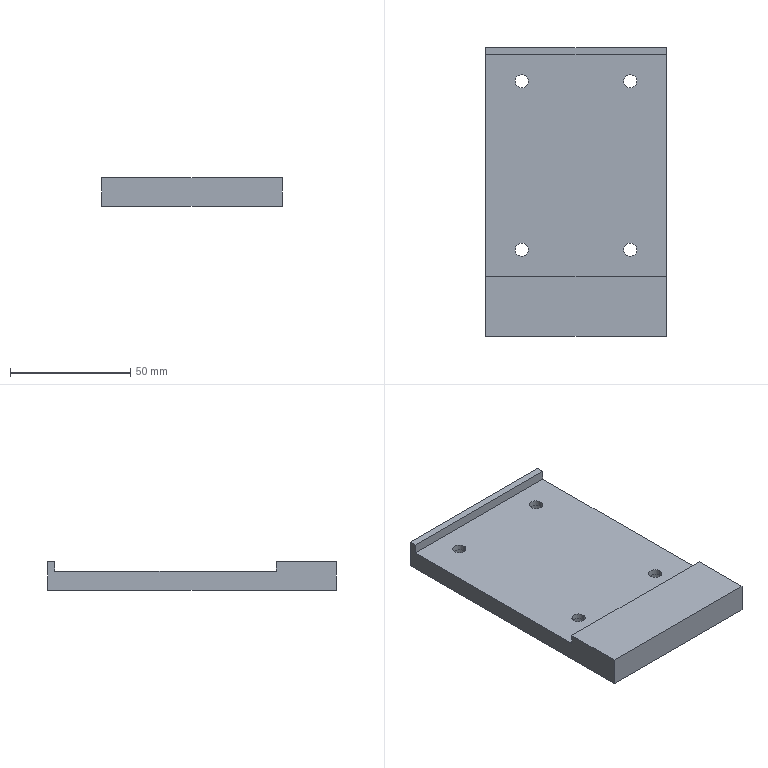Part | STEP file | 001-004-Feeding mechanism adapter plate | 1 solid | 30 faces | box 75 x 120 x 12 mm | volume 78391 mm3 | cylinder 16 | plane 14 | commonest cylinder face diameters 5.5 x8 10 x8